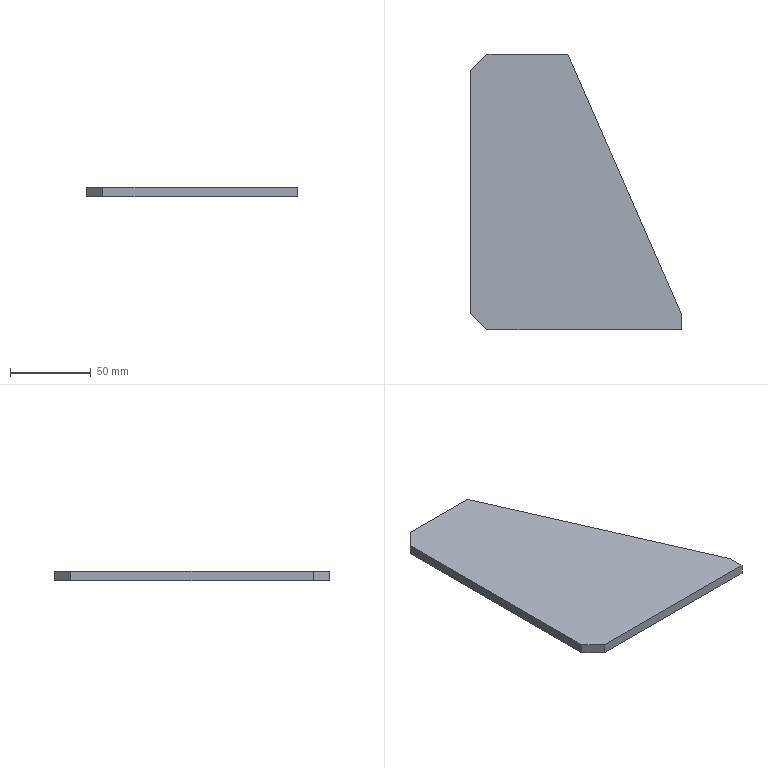Part | SolidWorks | features Chamfer 1, Extrusion 1 | 1 solid | 9 faces | box 130 x 170 x 6 mm | volume 98400 mm3 | plane 9
STEP:
#1=CARTESIAN_POINT('',(60.,170.,-3.));
#2=VERTEX_POINT('',#1);
#3=CARTESIAN_POINT('',(10.,170.,-3.));
#4=VERTEX_POINT('',#3);
#5=CARTESIAN_POINT('',(60.,170.,-3.));
#6=DIRECTION('',(-1.,0.,0.));
#7=VECTOR('',#6,1000.);
#8=LINE('',#5,#7);
#9=EDGE_CURVE('',#2,#4,#8,.T.);
#10=ORIENTED_EDGE('',*,*,#9,.T.);
#11=CARTESIAN_POINT('',(10.,170.,3.));
#12=VERTEX_POINT('',#11);
#13=CARTESIAN_POINT('',(10.,170.,3.));
#14=DIRECTION('',(0.,0.,1.));
#15=VECTOR('',#14,1000.);
#16=LINE('',#13,#15);
#17=EDGE_CURVE('',#4,#12,#16,.T.);
#18=ORIENTED_EDGE('',*,*,#17,.T.);
#19=CARTESIAN_POINT('',(60.,170.,3.));
#20=VERTEX_POINT('',#19);
#21=CARTESIAN_POINT('',(60.,170.,3.));
#22=DIRECTION('',(-1.,0.,0.));
#23=VECTOR('',#22,1000.);
#24=LINE('',#21,#23);
#25=EDGE_CURVE('',#20,#12,#24,.T.);
#26=ORIENTED_EDGE('',*,*,#25,.F.);
#27=CARTESIAN_POINT('',(60.,170.,3.));
#28=DIRECTION('',(0.,0.,-1.));
#29=VECTOR('',#28,1000.);
#30=LINE('',#27,#29);
#31=EDGE_CURVE('',#20,#2,#30,.T.);
#32=ORIENTED_EDGE('',*,*,#31,.T.);
#33=EDGE_LOOP('',(#10,#18,#26,#32));
#34=FACE_OUTER_BOUND('',#33,.T.);
#35=CARTESIAN_POINT('',(60.,170.,3.));
#36=DIRECTION('',(0.,-1.,0.));
#37=DIRECTION('',(0.,0.,-1.));
#38=AXIS2_PLACEMENT_3D('',#35,#36,#37);
#39=PLANE('',#38);
#40=ADVANCED_FACE('',(#34),#39,.F.);
#41=CARTESIAN_POINT('',(0.,160.,3.));
#42=VERTEX_POINT('',#41);
#43=CARTESIAN_POINT('',(0.,10.,3.));
#44=VERTEX_POINT('',#43);
#45=CARTESIAN_POINT('',(0.,170.,3.));
#46=DIRECTION('',(0.,-1.,0.));
#47=VECTOR('',#46,1000.);
#48=LINE('',#45,#47);
#49=EDGE_CURVE('',#42,#44,#48,.T.);
#50=ORIENTED_EDGE('',*,*,#49,.F.);
#51=CARTESIAN_POINT('',(0.,160.,-3.));
#52=VERTEX_POINT('',#51);
#53=CARTESIAN_POINT('',(0.,160.,3.));
#54=DIRECTION('',(0.,0.,-1.));
#55=VECTOR('',#54,1000.);
#56=LINE('',#53,#55);
#57=EDGE_CURVE('',#42,#52,#56,.T.);
#58=ORIENTED_EDGE('',*,*,#57,.T.);
#59=CARTESIAN_POINT('',(0.,10.,-3.));
#60=VERTEX_POINT('',#59);
#61=CARTESIAN_POINT('',(0.,170.,-3.));
#62=DIRECTION('',(0.,-1.,0.));
#63=VECTOR('',#62,1000.);
#64=LINE('',#61,#63);
#65=EDGE_CURVE('',#52,#60,#64,.T.);
#66=ORIENTED_EDGE('',*,*,#65,.T.);
#67=CARTESIAN_POINT('',(0.,10.,3.));
#68=DIRECTION('',(0.,0.,1.));
#69=VECTOR('',#68,1000.);
#70=LINE('',#67,#69);
#71=EDGE_CURVE('',#60,#44,#70,.T.);
#72=ORIENTED_EDGE('',*,*,#71,.T.);
#73=EDGE_LOOP('',(#50,#58,#66,#72));
#74=FACE_OUTER_BOUND('',#73,.T.);
#75=CARTESIAN_POINT('',(0.,170.,3.));
#76=DIRECTION('',(1.,0.,0.));
#77=DIRECTION('',(0.,1.,0.));
#78=AXIS2_PLACEMENT_3D('',#75,#76,#77);
#79=PLANE('',#78);
#80=ADVANCED_FACE('',(#74),#79,.F.);
#81=CARTESIAN_POINT('',(10.,0.,3.));
#82=VERTEX_POINT('',#81);
#83=CARTESIAN_POINT('',(130.,0.,3.));
#84=VERTEX_POINT('',#83);
#85=CARTESIAN_POINT('',(0.,0.,3.));
#86=DIRECTION('',(1.,0.,0.));
#87=VECTOR('',#86,1000.);
#88=LINE('',#85,#87);
#89=EDGE_CURVE('',#82,#84,#88,.T.);
#90=ORIENTED_EDGE('',*,*,#89,.F.);
#91=CARTESIAN_POINT('',(10.,0.,-3.));
#92=VERTEX_POINT('',#91);
#93=CARTESIAN_POINT('',(10.,0.,3.));
#94=DIRECTION('',(0.,0.,-1.));
#95=VECTOR('',#94,1000.);
#96=LINE('',#93,#95);
#97=EDGE_CURVE('',#82,#92,#96,.T.);
#98=ORIENTED_EDGE('',*,*,#97,.T.);
#99=CARTESIAN_POINT('',(130.,0.,-3.));
#100=VERTEX_POINT('',#99);
#101=CARTESIAN_POINT('',(0.,0.,-3.));
#102=DIRECTION('',(1.,0.,0.));
#103=VECTOR('',#102,1000.);
#104=LINE('',#101,#103);
#105=EDGE_CURVE('',#92,#100,#104,.T.);
#106=ORIENTED_EDGE('',*,*,#105,.T.);
#107=CARTESIAN_POINT('',(130.,0.,3.));
#108=DIRECTION('',(0.,0.,-1.));
#109=VECTOR('',#108,1000.);
#110=LINE('',#107,#109);
#111=EDGE_CURVE('',#84,#100,#110,.T.);
#112=ORIENTED_EDGE('',*,*,#111,.F.);
#113=EDGE_LOOP('',(#90,#98,#106,#112));
#114=FACE_OUTER_BOUND('',#113,.T.);
#115=CARTESIAN_POINT('',(0.,0.,3.));
#116=DIRECTION('',(0.,1.,0.));
#117=DIRECTION('',(0.,0.,1.));
#118=AXIS2_PLACEMENT_3D('',#115,#116,#117);
#119=PLANE('',#118);
#120=ADVANCED_FACE('',(#114),#119,.F.);
#121=CARTESIAN_POINT('',(130.,10.,-3.));
#122=VERTEX_POINT('',#121);
#123=CARTESIAN_POINT('',(130.,0.,-3.));
#124=DIRECTION('',(0.,1.,0.));
#125=VECTOR('',#124,1000.);
#126=LINE('',#123,#125);
#127=EDGE_CURVE('',#100,#122,#126,.T.);
#128=ORIENTED_EDGE('',*,*,#127,.T.);
#129=CARTESIAN_POINT('',(130.,10.,3.));
#130=VERTEX_POINT('',#129);
#131=CARTESIAN_POINT('',(130.,10.,3.));
#132=DIRECTION('',(0.,0.,-1.));
#133=VECTOR('',#132,1000.);
#134=LINE('',#131,#133);
#135=EDGE_CURVE('',#130,#122,#134,.T.);
#136=ORIENTED_EDGE('',*,*,#135,.F.);
#137=CARTESIAN_POINT('',(130.,0.,3.));
#138=DIRECTION('',(0.,1.,0.));
#139=VECTOR('',#138,1000.);
#140=LINE('',#137,#139);
#141=EDGE_CURVE('',#84,#130,#140,.T.);
#142=ORIENTED_EDGE('',*,*,#141,.F.);
#143=ORIENTED_EDGE('',*,*,#111,.T.);
#144=EDGE_LOOP('',(#128,#136,#142,#143));
#145=FACE_OUTER_BOUND('',#144,.T.);
#146=CARTESIAN_POINT('',(130.,0.,3.));
#147=DIRECTION('',(-1.,0.,0.));
#148=DIRECTION('',(0.,0.,1.));
#149=AXIS2_PLACEMENT_3D('',#146,#147,#148);
#150=PLANE('',#149);
#151=ADVANCED_FACE('',(#145),#150,.F.);
#152=CARTESIAN_POINT('',(130.,10.,-3.));
#153=DIRECTION('',(-0.4008,0.9162,0.));
#154=VECTOR('',#153,1000.);
#155=LINE('',#152,#154);
#156=EDGE_CURVE('',#122,#2,#155,.T.);
#157=ORIENTED_EDGE('',*,*,#156,.T.);
#158=ORIENTED_EDGE('',*,*,#31,.F.);
#159=CARTESIAN_POINT('',(130.,10.,3.));
#160=DIRECTION('',(-0.4008,0.9162,0.));
#161=VECTOR('',#160,1000.);
#162=LINE('',#159,#161);
#163=EDGE_CURVE('',#130,#20,#162,.T.);
#164=ORIENTED_EDGE('',*,*,#163,.F.);
#165=ORIENTED_EDGE('',*,*,#135,.T.);
#166=EDGE_LOOP('',(#157,#158,#164,#165));
#167=FACE_OUTER_BOUND('',#166,.T.);
#168=CARTESIAN_POINT('',(130.,10.,3.));
#169=DIRECTION('',(-0.9162,-0.4008,0.));
#170=DIRECTION('',(0.4008,-0.9162,0.));
#171=AXIS2_PLACEMENT_3D('',#168,#169,#170);
#172=PLANE('',#171);
#173=ADVANCED_FACE('',(#167),#172,.F.);
#174=ORIENTED_EDGE('',*,*,#25,.T.);
#175=CARTESIAN_POINT('',(-80.,80.,3.));
#176=DIRECTION('',(-0.7071,-0.7071,0.));
#177=VECTOR('',#176,1000.);
#178=LINE('',#175,#177);
#179=EDGE_CURVE('',#12,#42,#178,.T.);
#180=ORIENTED_EDGE('',*,*,#179,.T.);
#181=ORIENTED_EDGE('',*,*,#49,.T.);
#182=CARTESIAN_POINT('',(5.,5.,3.));
#183=DIRECTION('',(0.7071,-0.7071,0.));
#184=VECTOR('',#183,1000.);
#185=LINE('',#182,#184);
#186=EDGE_CURVE('',#44,#82,#185,.T.);
#187=ORIENTED_EDGE('',*,*,#186,.T.);
#188=ORIENTED_EDGE('',*,*,#89,.T.);
#189=ORIENTED_EDGE('',*,*,#141,.T.);
#190=ORIENTED_EDGE('',*,*,#163,.T.);
#191=EDGE_LOOP('',(#174,#180,#181,#187,#188,#189,#190));
#192=FACE_OUTER_BOUND('',#191,.T.);
#193=CARTESIAN_POINT('',(0.,0.,3.));
#194=DIRECTION('',(0.,0.,1.));
#195=DIRECTION('',(1.,0.,0.));
#196=AXIS2_PLACEMENT_3D('',#193,#194,#195);
#197=PLANE('',#196);
#198=ADVANCED_FACE('',(#192),#197,.T.);
#199=ORIENTED_EDGE('',*,*,#65,.F.);
#200=CARTESIAN_POINT('',(0.,160.,-3.));
#201=DIRECTION('',(0.7071,0.7071,0.));
#202=VECTOR('',#201,1000.);
#203=LINE('',#200,#202);
#204=EDGE_CURVE('',#52,#4,#203,.T.);
#205=ORIENTED_EDGE('',*,*,#204,.T.);
#206=ORIENTED_EDGE('',*,*,#9,.F.);
#207=ORIENTED_EDGE('',*,*,#156,.F.);
#208=ORIENTED_EDGE('',*,*,#127,.F.);
#209=ORIENTED_EDGE('',*,*,#105,.F.);
#210=CARTESIAN_POINT('',(10.,0.,-3.));
#211=DIRECTION('',(-0.7071,0.7071,0.));
#212=VECTOR('',#211,1000.);
#213=LINE('',#210,#212);
#214=EDGE_CURVE('',#92,#60,#213,.T.);
#215=ORIENTED_EDGE('',*,*,#214,.T.);
#216=EDGE_LOOP('',(#199,#205,#206,#207,#208,#209,#215));
#217=FACE_OUTER_BOUND('',#216,.T.);
#218=CARTESIAN_POINT('',(0.,0.,-3.));
#219=DIRECTION('',(0.,0.,1.));
#220=DIRECTION('',(1.,0.,0.));
#221=AXIS2_PLACEMENT_3D('',#218,#219,#220);
#222=PLANE('',#221);
#223=ADVANCED_FACE('',(#217),#222,.F.);
#224=ORIENTED_EDGE('',*,*,#179,.F.);
#225=ORIENTED_EDGE('',*,*,#17,.F.);
#226=ORIENTED_EDGE('',*,*,#204,.F.);
#227=ORIENTED_EDGE('',*,*,#57,.F.);
#228=EDGE_LOOP('',(#224,#225,#226,#227));
#229=FACE_OUTER_BOUND('',#228,.T.);
#230=CARTESIAN_POINT('',(0.,160.,3.));
#231=DIRECTION('',(0.7071,-0.7071,0.));
#232=DIRECTION('',(0.,0.,-1.));
#233=AXIS2_PLACEMENT_3D('',#230,#231,#232);
#234=PLANE('',#233);
#235=ADVANCED_FACE('',(#229),#234,.F.);
#236=ORIENTED_EDGE('',*,*,#186,.F.);
#237=ORIENTED_EDGE('',*,*,#71,.F.);
#238=ORIENTED_EDGE('',*,*,#214,.F.);
#239=ORIENTED_EDGE('',*,*,#97,.F.);
#240=EDGE_LOOP('',(#236,#237,#238,#239));
#241=FACE_OUTER_BOUND('',#240,.T.);
#242=CARTESIAN_POINT('',(10.,0.,3.));
#243=DIRECTION('',(0.7071,0.7071,0.));
#244=DIRECTION('',(0.,0.,-1.));
#245=AXIS2_PLACEMENT_3D('',#242,#243,#244);
#246=PLANE('',#245);
#247=ADVANCED_FACE('',(#241),#246,.F.);
#248=CLOSED_SHELL('',(#40,#80,#120,#151,#173,#198,#223,#235,#247));
#249=MANIFOLD_SOLID_BREP('',#248);
#250=CARTESIAN_POINT('',(0.,0.,0.));
#251=DIRECTION('',(0.,0.,1.));
#252=DIRECTION('',(1.,0.,0.));
#253=AXIS2_PLACEMENT_3D('',#250,#251,#252);
#254=(LENGTH_UNIT()NAMED_UNIT(*)SI_UNIT(.MILLI.,.METRE.));
#255=UNCERTAINTY_MEASURE_WITH_UNIT(LENGTH_MEASURE(0.00001),#254,'','');
#256=(NAMED_UNIT(*)PLANE_ANGLE_UNIT()SI_UNIT($,.RADIAN.));
#257=(NAMED_UNIT(*)SI_UNIT($,.STERADIAN.)SOLID_ANGLE_UNIT());
#258=(GEOMETRIC_REPRESENTATION_CONTEXT(3)GLOBAL_UNCERTAINTY_ASSIGNED_CONTEXT((#255))GLOBAL_UNIT_ASSIGNED_CONTEXT((#254,#256,#257))REPRESENTATION_CONTEXT('',''));
#259=ADVANCED_BREP_SHAPE_REPRESENTATION('',(#249,#253),#258);